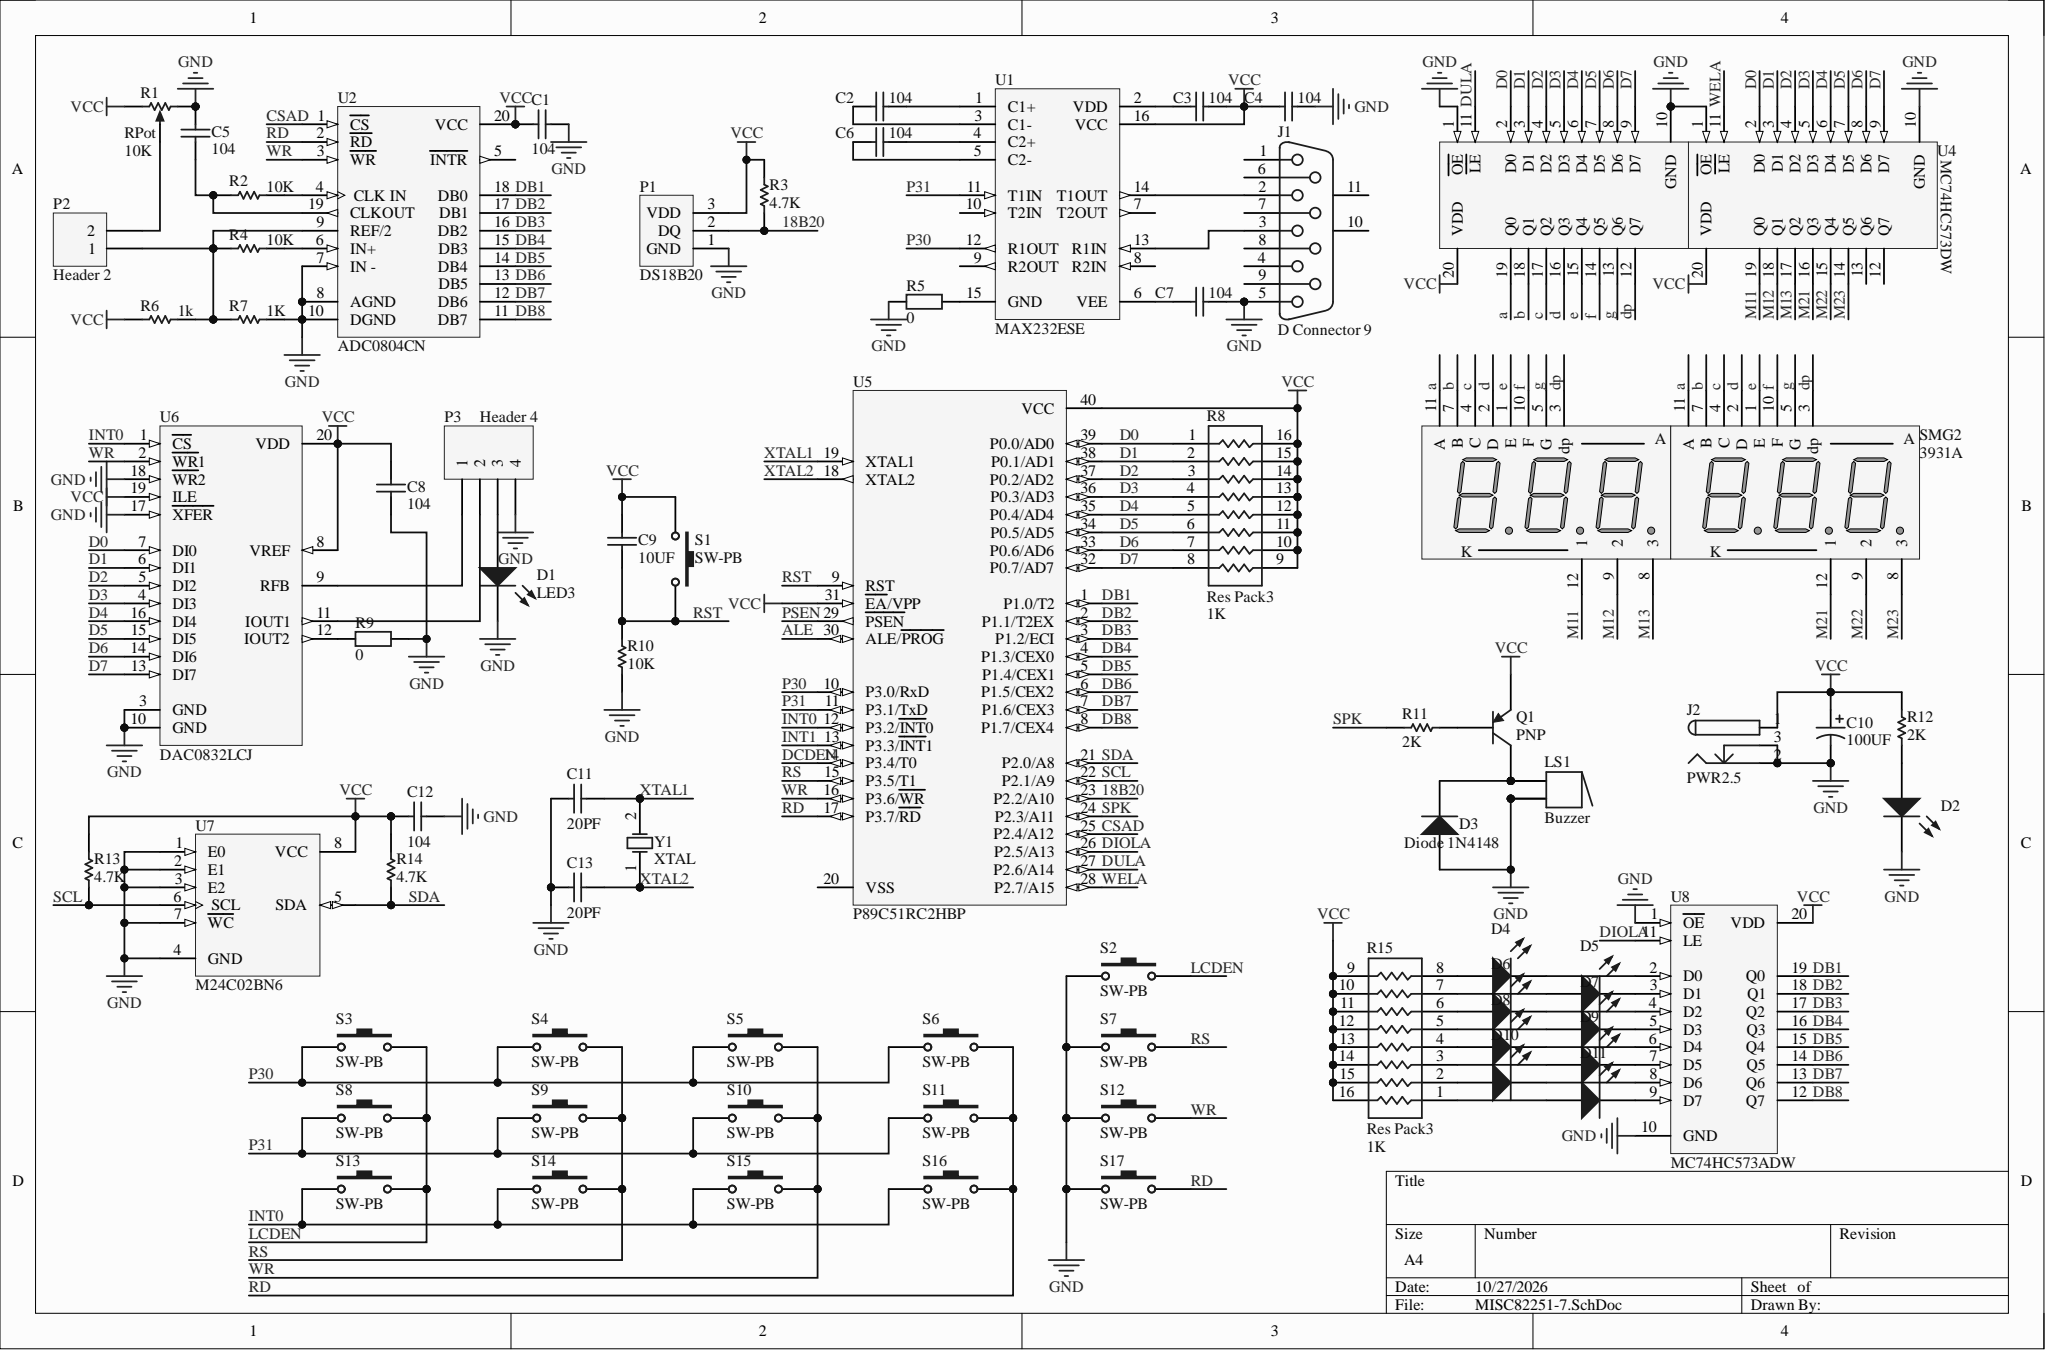Circuit board | Altium Designer | 74 parts | 87 nets
Bill of materials:
Comment,Description,Designator,Footprint,LibRef,Quantity
"104","Capacitor","C1, C2, C3, C4, C5, C6, C7, C8, C12","RAD-0.3","Cap","9"
"10UF","Capacitor","C9","RAD-0.3","Cap","1"
"100UF","Polarized Capacitor (Radial)","C10","RB7.6-15","Cap Pol1","1"
"20PF","Capacitor","C11, C13","RAD-0.1","Cap","2"
"LED3","Typical BLUE SiC LED","D1, D2, D4, D5, D6, D7, D8, D9, D10, D11","3.5X2.8X1.9","LED3","10"
"Diode 1N4148","High Conductance Fast Diode","D3","DO-35","Diode 1N4148","1"
"D Connector 9","Receptacle Assembly, 9 Position, Right Angle","J1","DSUB1.385-2H9","D Connector 9","1"
"PWR2.5","","J2","DC-002","DC_Socket","1"
"Buzzer","Magnetic Transducer Buzzer","LS1","ABSM-1574","Buzzer","1"
"DS18B20","Header, 3-Pin","P1","HDR1X3","Header 3","1"
"Header 2","Header, 2-Pin","P2","HDR1X2","Header 2","1"
"Header 4","Header, 4-Pin","P3","HDR1X4","Header 4","1"
"PNP","PNP Bipolar Transistor","Q1","SOT-23B_N","PNP","1"
"RPot","Potentiometer","R1","VR5","RPot","1"
"10K","Resistor","R2, R4, R10","AXIAL-0.3","Res1","3"
"4.7K","Resistor","R3, R13, R14","AXIAL-0.3","Res1","3"
"0","Resistor","R5, R9","AXIAL-0.4","Res2","2"
"1k","Resistor","R6, R7","AXIAL-0.3","Res1","2"
"Res Pack3","Isolated Resistor Network","R8, R15","SO-16_N","Res Pack3","2"
"2K","Resistor","R11, R12","AXIAL-0.3","Res1","2"
"SW-PB","Switch","S1, S2, S3, S4, S5, S6, S7, S8, S9, S10, S11, S12, S13, S14, S15, S16, S17","SPST-2","SW-PB","17"
"3931A","0.39 inch 3-digit common-cathode LED display","SMG1, SMG2","SMG 0.39-3P","3931A","2"
"MAX232ESE","+5V Powered, Multi-Channel RS-232 Driver/Receiver","U1","DIP16","MAX232ESE","1"
"ADC0804CN","8-Bit Analog-to-Digital Converter with Differential Inputs","U2","N020","ADC0804CN","1"
"MC74HC573DW","Octal 3-State Non-Inverting Transparent Latch","U3, U4","751D-03","MC74HC573DW","2"
"P89C51RC2HBP","80C51 8-Bit Flash Microcontroller Family, 32 kB ISP/IAP Flash with 512 B RAM.","U5","SOT129-1","P89C51RC2HBP","1"
"DAC0832LCJ","8-Bit uP-Compatible, Double-Buffered Digital-to-Analog Converter","U6","J20A","DAC0832LCJ","1"
"M24C02BN6","2Kbit Serial IIC Bus EEPROM","U7","PSDIP8A","M24C02BN6","1"
"MC74HC573ADW","Octal 3-State Non-Inverting Transparent Latch","U8","751D-05","MC74HC573ADW","1"
"XTAL","Crystal Oscillator","Y1","R38","XTAL","1"
Netlist (Protel format):
[
C1
RAD-0.3
104



]
[
C2
RAD-0.3
104



]
[
C3
RAD-0.3
104



]
[
C4
RAD-0.3
104



]
[
C5
RAD-0.3
104



]
[
C6
RAD-0.3
104



]
[
C7
RAD-0.3
104



]
[
C8
RAD-0.3
104



]
[
C9
RAD-0.3
10UF



]
[
C10
RB7.6-15
100UF



]
[
C11
RAD-0.1
20PF



]
[
C12
RAD-0.3
104



]
[
C13
RAD-0.1
20PF



]
[
D1
3.5X2.8X1.9
LED3



]
[
D2
3.5X2.8X1.9
LED3



]
[
D3
DO-35
Diode 1N4148



]
[
D4
3.5X2.8X1.9
LED3



]
[
D5
3.5X2.8X1.9
LED3



]
[
D6
3.5X2.8X1.9
LED3



]
[
D7
3.5X2.8X1.9
LED3



]
[
D8
3.5X2.8X1.9
LED3



]
[
D9
3.5X2.8X1.9
LED3



]
[
D10
3.5X2.8X1.9
LED3



]
[
D11
3.5X2.8X1.9
LED3



]
[
J1
DSUB1.385-2H9
D Connector 9



]
[
J2
DC-002
PWR2.5



]
[
LS1
ABSM-1574
Buzzer



]
[
P1
HDR1X3
DS18B20



]
[
P2
HDR1X2
Header 2



]
[
P3
HDR1X4
Header 4



]
[
Q1
SOT-23B_N
PNP



]
[
R1
VR5
RPot



]
[
R2
AXIAL-0.3
10K



]
[
R3
AXIAL-0.3
4.7K



]
[
R4
AXIAL-0.3
10K



]
[
R5
AXIAL-0.4
0



]
[
R6
AXIAL-0.3
1k



]
[
R7
AXIAL-0.3
1K



]
[
R8
SO-16_N
Res Pack3



]
[
R9
AXIAL-0.4
0



]
[
R10
AXIAL-0.3
10K



]
[
R11
AXIAL-0.3
2K



]
[
R12
AXIAL-0.3
2K



]
[
R13
AXIAL-0.3
4.7K



]
[
R14
AXIAL-0.3
4.7K



]
[
R15
SO-16_N
Res Pack3



]
[
S1
SPST-2
SW-PB



]
[
S2
SPST-2
SW-PB



]
[
S3
SPST-2
SW-PB



]
[
S4
SPST-2
SW-PB



]
[
S5
SPST-2
SW-PB



]
[
S6
SPST-2
SW-PB



]
[
S7
SPST-2
SW-PB



]
[
S8
SPST-2
SW-PB



]
[
S9
SPST-2
SW-PB



]
[
S10
SPST-2
SW-PB



]
[
S11
SPST-2
SW-PB



]
[
S12
SPST-2
SW-PB



]
[
S13
SPST-2
SW-PB



]
[
S14
SPST-2
SW-PB



]
[
S15
SPST-2
SW-PB



]
[
S16
SPST-2
SW-PB



]
[
S17
SPST-2
SW-PB



]
[
SMG1
SMG 0.39-3P
3931A



]
[
SMG2
SMG 0.39-3P
3931A



]
[
U1
DIP16
MAX232ESE



]
[
U2
N020
ADC0804CN



]
[
U3
751D-03
MC74HC573DW



]
[
U4
751D-03
MC74HC573DW



]
[
U5
SOT129-1
P89C51RC2HBP



]
[
U6
J20A
DAC0832LCJ



]
[
U7
PSDIP8A
M24C02BN6



]
[
U8
751D-05
MC74HC573ADW



]
[
Y1
R38
XTAL



]
(
XTAL2
C13-1
U5-18
Y1-1
)
(
XTAL1
C11-1
U5-19
Y1-2
)
(
WR
S5-2
S10-2
S12-2
S15-2
U2-3
U5-16
U6-2
)
(
WELA
U4-11
U5-28
)
(
VCC
C1-2
C3-1
C4-2
C8-1
C9-2
C10-1
C12-1
J2-1
P1-3
Q1-3
R1-1
R3-2
R6-1
R8-9
R8-10
R8-11
R8-12
R8-13
R8-14
R8-15
R8-16
R12-2
R13-2
R14-2
R15-9
R15-10
R15-11
R15-12
R15-13
R15-14
R15-15
R15-16
S1-1
U1-16
U2-20
U3-20
U4-20
U5-31
U5-40
U6-8
U6-19
U6-20
U7-8
U8-20
)
(
SPK
R11-2
U5-24
)
(
SDA
R14-1
U5-21
U7-5
)
(
SCL
R13-1
U5-22
U7-6
)
(
RST
C9-1
R10-2
S1-2
U5-9
)
(
RS
S4-2
S7-2
S9-2
S14-2
U5-15
)
(
RD
S6-2
S11-2
S16-2
S17-2
U2-2
U5-17
)
(
P31
S8-1
S9-1
S10-1
S11-1
U1-11
U5-11
)
(
P30
S3-1
S4-1
S5-1
S6-1
U1-12
U5-10
)
(
NetR9_1
R9-1
U6-12
)
(
NetR5_2
R5-2
U1-15
)
(
NetR4_2
R4-2
U2-6
)
(
NetR2_2
R2-2
U2-4
)
(
NetQ1_2
Q1-2
R11-1
)
(
NetP3_2
P3-2
U6-11
)
(
NetP3_1
P3-1
U6-9
)
(
NetP2_2
P2-2
R1-3
)
(
NetP2_1
P2-1
R4-1
R6-2
R7-1
U2-9
)
(
NetJ1_3
J1-3
U1-13
)
(
NetJ1_2
J1-2
U1-14
)
(
NetD11_2
D11-2
U8-9
)
(
NetD11_1
D11-1
R15-1
)
(
NetD10_2
D10-2
U8-8
)
(
NetD10_1
D10-1
R15-2
)
(
NetD9_2
D9-2
U8-7
)
(
NetD9_1
D9-1
R15-3
)
(
NetD8_2
D8-2
U8-6
)
(
NetD8_1
D8-1
R15-4
)
(
NetD7_2
D7-2
U8-5
)
(
NetD7_1
D7-1
R15-5
)
(
NetD6_2
D6-2
U8-4
)
(
NetD6_1
D6-1
R15-6
)
(
NetD5_2
D5-2
U8-3
)
(
NetD5_1
D5-1
R15-7
)
(
NetD4_2
D4-2
U8-2
)
(
NetD4_1
D4-1
R15-8
)
(
NetD3_2
D3-2
LS1-1
LS1-1A
Q1-1
)
(
NetD2_1
D2-1
R12-1
)
(
NetD1_1
D1-1
P3-3
)
(
NetC7_2
C7-2
U1-6
)
(
NetC6_2
C6-2
U1-5
)
(
NetC6_1
C6-1
U1-4
)
(
NetC5_1
C5-1
R2-1
U2-19
)
(
NetC3_2
C3-2
U1-2
)
(
NetC2_2
C2-2
U1-3
)
(
NetC2_1
C2-1
U1-1
)
(
M23
SMG2-8
U4-14
)
(
M22
SMG2-9
U4-15
)
(
M21
SMG2-12
U4-16
)
(
M13
SMG1-8
U4-17
)
(
M12
SMG1-9
U4-18
)
(
M11
SMG1-12
U4-19
)
(
LCDEN
S2-2
S3-2
S8-2
S13-2
)
(
INT0
S13-1
S14-1
S15-1
S16-1
U5-12
U6-1
)
(
GND
C1-1
C4-1
C5-2
C7-1
C8-2
C10-2
C11-2
C12-2
C13-2
D1-2
D2-2
D3-1
J1-5
J2-2
J2-3
LS1-2
LS1-2A
P1-1
P3-4
R1-2
R5-1
R7-2
R9-2
R10-1
S2-1
S7-1
S12-1
S17-1
U2-7
U2-8
U2-10
U3-1
U3-10
U4-1
U4-10
U6-3
U6-10
U6-17
U6-18
U7-1
U7-2
U7-3
U7-4
U7-7
U8-1
U8-10
)
(
g
SMG1-5
SMG2-5
U3-13
)
(
f
SMG1-10
SMG2-10
U3-14
)
(
e
SMG1-1
SMG2-1
U3-15
)
(
DULA
U3-11
U5-27
)
(
dp
SMG1-3
SMG2-3
U3-12
)
(
DIOLA
U5-26
U8-11
)
(
DB8
U2-11
U5-8
U8-12
)
(
DB7
U2-12
U5-7
U8-13
)
(
DB6
U2-13
U5-6
U8-14
)
(
DB5
U2-14
U5-5
U8-15
)
(
DB4
U2-15
U5-4
U8-16
)
(
DB3
U2-16
U5-3
U8-17
)
(
DB2
U2-17
U5-2
U8-18
)
(
DB1
U2-18
U5-1
U8-19
)
(
D7
R8-8
U3-9
U4-9
U5-32
U6-13
)
(
D6
R8-7
U3-8
U4-8
U5-33
U6-14
)
(
D5
R8-6
U3-7
U4-7
U5-34
U6-15
)
(
D4
R8-5
U3-6
U4-6
U5-35
U6-16
)
(
D3
R8-4
U3-5
U4-5
U5-36
U6-4
)
(
D2
R8-3
U3-4
U4-4
U5-37
U6-5
)
(
D1
R8-2
U3-3
U4-3
U5-38
U6-6
)
(
D0
R8-1
U3-2
U4-2
U5-39
U6-7
)
(
d
SMG1-2
SMG2-2
U3-16
)
(
CSAD
U2-1
U5-25
)
(
c
SMG1-4
SMG2-4
U3-17
)
(
b
SMG1-7
SMG2-7
U3-18
)
(
a
SMG1-11
SMG2-11
U3-19
)
(
18B20
P1-2
R3-1
U5-23
)